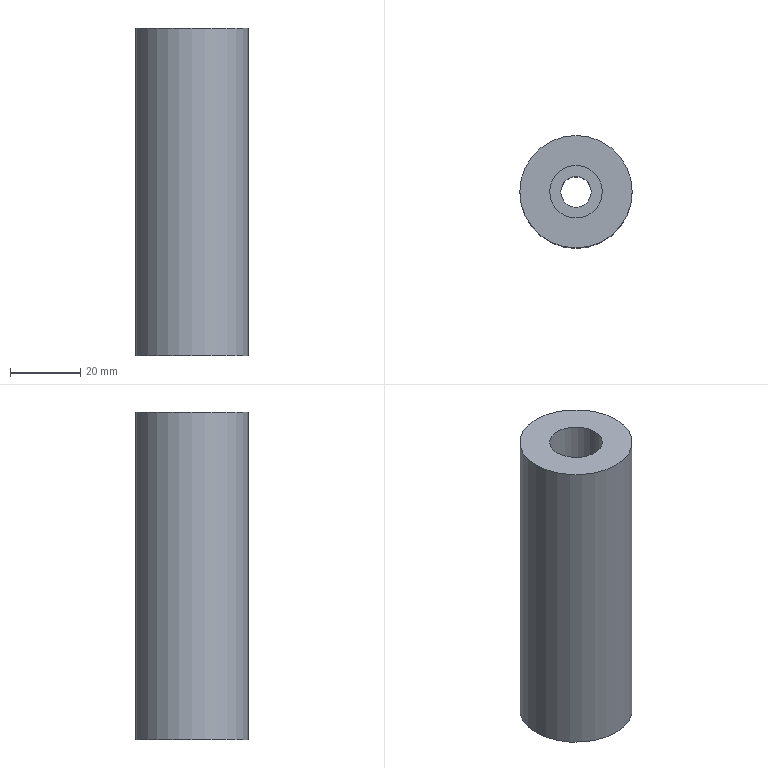Part | STEP file | 1_id1238_x_t | 1 solid | 6 faces | box 32 x 32 x 93.24 mm | volume 66514 mm3 | cylinder 3 | plane 3 | commonest cylinder face diameters 8.7 x1 15 x1 32 x1
STEP:
#1=CARTESIAN_POINT('',(0.,0.,0.));
#2=DIRECTION('',(0.,0.,1.));
#3=DIRECTION('',(1.,0.,0.));
#4=AXIS2_PLACEMENT_3D('',#1,#2,#3);
#5=CARTESIAN_POINT('',(906.425,64.5,-90.));
#6=VERTEX_POINT('',#5);
#7=CARTESIAN_POINT('',(874.425,64.5,-90.));
#8=VERTEX_POINT('',#7);
#9=CARTESIAN_POINT('',(890.425,64.5,-90.));
#10=DIRECTION('',(0.,0.,-1.));
#11=DIRECTION('',(-1.,0.,0.));
#12=AXIS2_PLACEMENT_3D('',#9,#10,#11);
#13=CIRCLE('',#12,16.);
#14=CARTESIAN_POINT('',(890.425,64.5,-46.76));
#15=DIRECTION('',(0.,0.,-1.));
#16=DIRECTION('',(1.,0.,0.));
#17=AXIS2_PLACEMENT_3D('',#14,#15,#16);
#18=CYLINDRICAL_SURFACE('',#17,16.);
#19=CARTESIAN_POINT('',(-3.142,43.24));
#20=DIRECTION('',(1.,0.));
#21=VECTOR('',#20,1.);
#22=LINE('',#19,#21);
#23=(GEOMETRIC_REPRESENTATION_CONTEXT(2)PARAMETRIC_REPRESENTATION_CONTEXT()REPRESENTATION_CONTEXT('',''));
#24=DEFINITIONAL_REPRESENTATION('',(#22),#23);
#25=PCURVE('',#18,#24);
#26=CARTESIAN_POINT('',(1119.226,213.819,-90.));
#27=DIRECTION('',(0.,0.,-1.));
#28=DIRECTION('',(0.,1.,0.));
#29=AXIS2_PLACEMENT_3D('',#26,#27,#28);
#30=PLANE('',#29);
#31=CARTESIAN_POINT('',(-149.319,-228.801));
#32=DIRECTION('',(0.,-1.));
#33=AXIS2_PLACEMENT_2D('',#31,#32);
#34=CIRCLE('',#33,16.);
#35=(GEOMETRIC_REPRESENTATION_CONTEXT(2)PARAMETRIC_REPRESENTATION_CONTEXT()REPRESENTATION_CONTEXT('',''));
#36=DEFINITIONAL_REPRESENTATION('',(#34),#35);
#37=PCURVE('',#30,#36);
#38=SURFACE_CURVE('',#13,(#25,#37),.PCURVE_S1.);
#39=EDGE_CURVE('',#6,#8,#38,.T.);
#40=ORIENTED_EDGE('',*,*,#39,.F.);
#41=CARTESIAN_POINT('',(906.425,64.5,3.24));
#42=VERTEX_POINT('',#41);
#43=CARTESIAN_POINT('',(906.425,64.5,3.24));
#44=CARTESIAN_POINT('',(906.425,64.5,-90.));
#45=B_SPLINE_CURVE_WITH_KNOTS('',1,(#43,#44),.UNSPECIFIED.,.F.,.F.,(2,2),(-50.,43.24),.PIECEWISE_BEZIER_KNOTS.);
#46=CARTESIAN_POINT('',(0.,0.));
#47=DIRECTION('',(0.,1.));
#48=VECTOR('',#47,1.);
#49=LINE('',#46,#48);
#50=(GEOMETRIC_REPRESENTATION_CONTEXT(2)PARAMETRIC_REPRESENTATION_CONTEXT()REPRESENTATION_CONTEXT('',''));
#51=DEFINITIONAL_REPRESENTATION('',(#49),#50);
#52=PCURVE('',#18,#51);
#53=CARTESIAN_POINT('',(6.283,0.));
#54=DIRECTION('',(0.,1.));
#55=VECTOR('',#54,1.);
#56=LINE('',#53,#55);
#57=(GEOMETRIC_REPRESENTATION_CONTEXT(2)PARAMETRIC_REPRESENTATION_CONTEXT()REPRESENTATION_CONTEXT('',''));
#58=DEFINITIONAL_REPRESENTATION('',(#56),#57);
#59=PCURVE('',#18,#58);
#60=SEAM_CURVE('',#45,(#52,#59),.PCURVE_S1.);
#61=EDGE_CURVE('',#42,#6,#60,.T.);
#62=ORIENTED_EDGE('',*,*,#61,.F.);
#63=CARTESIAN_POINT('',(890.425,64.5,3.24));
#64=DIRECTION('',(0.,0.,1.));
#65=DIRECTION('',(1.,0.,0.));
#66=AXIS2_PLACEMENT_3D('',#63,#64,#65);
#67=CIRCLE('',#66,16.);
#68=CARTESIAN_POINT('',(6.283,-50.));
#69=DIRECTION('',(-1.,0.));
#70=VECTOR('',#69,1.);
#71=LINE('',#68,#70);
#72=(GEOMETRIC_REPRESENTATION_CONTEXT(2)PARAMETRIC_REPRESENTATION_CONTEXT()REPRESENTATION_CONTEXT('',''));
#73=DEFINITIONAL_REPRESENTATION('',(#71),#72);
#74=PCURVE('',#18,#73);
#75=CARTESIAN_POINT('',(890.425,64.5,3.24));
#76=DIRECTION('',(0.,0.,-1.));
#77=DIRECTION('',(-1.,0.,0.));
#78=AXIS2_PLACEMENT_3D('',#75,#76,#77);
#79=PLANE('',#78);
#80=CARTESIAN_POINT('',(-16.,0.));
#81=CARTESIAN_POINT('',(-16.,27.713));
#82=CARTESIAN_POINT('',(8.,13.856));
#83=CARTESIAN_POINT('',(32.,0.));
#84=CARTESIAN_POINT('',(8.,-13.856));
#85=CARTESIAN_POINT('',(-16.,-27.713));
#86=CARTESIAN_POINT('',(-16.,0.));
#87=(BOUNDED_CURVE()B_SPLINE_CURVE(2,(#80,#81,#82,#83,#84,#85,#86),.UNSPECIFIED.,.T.,.F.)B_SPLINE_CURVE_WITH_KNOTS((1,2,2,2,2,1),(-2.094,0.,2.094,4.189,6.283,8.378),.UNSPECIFIED.)CURVE()GEOMETRIC_REPRESENTATION_ITEM()RATIONAL_B_SPLINE_CURVE((1.,0.5,1.,0.5,1.,0.5,1.))REPRESENTATION_ITEM(''));
#88=(GEOMETRIC_REPRESENTATION_CONTEXT(2)PARAMETRIC_REPRESENTATION_CONTEXT()REPRESENTATION_CONTEXT('',''));
#89=DEFINITIONAL_REPRESENTATION('',(#87),#88);
#90=PCURVE('',#79,#89);
#91=SURFACE_CURVE('',#67,(#74,#90),.PCURVE_S1.);
#92=EDGE_CURVE('',#42,#42,#91,.T.);
#93=ORIENTED_EDGE('',*,*,#92,.F.);
#94=ORIENTED_EDGE('',*,*,#61,.T.);
#95=CARTESIAN_POINT('',(890.425,64.5,-90.));
#96=DIRECTION('',(0.,0.,-1.));
#97=DIRECTION('',(-1.,0.,0.));
#98=AXIS2_PLACEMENT_3D('',#95,#96,#97);
#99=CIRCLE('',#98,16.);
#100=CARTESIAN_POINT('',(3.142,43.24));
#101=DIRECTION('',(1.,0.));
#102=VECTOR('',#101,1.);
#103=LINE('',#100,#102);
#104=(GEOMETRIC_REPRESENTATION_CONTEXT(2)PARAMETRIC_REPRESENTATION_CONTEXT()REPRESENTATION_CONTEXT('',''));
#105=DEFINITIONAL_REPRESENTATION('',(#103),#104);
#106=PCURVE('',#18,#105);
#107=CARTESIAN_POINT('',(-149.319,-228.801));
#108=DIRECTION('',(0.,-1.));
#109=AXIS2_PLACEMENT_2D('',#107,#108);
#110=CIRCLE('',#109,16.);
#111=(GEOMETRIC_REPRESENTATION_CONTEXT(2)PARAMETRIC_REPRESENTATION_CONTEXT()REPRESENTATION_CONTEXT('',''));
#112=DEFINITIONAL_REPRESENTATION('',(#110),#111);
#113=PCURVE('',#30,#112);
#114=SURFACE_CURVE('',#99,(#106,#113),.PCURVE_S1.);
#115=EDGE_CURVE('',#8,#6,#114,.T.);
#116=ORIENTED_EDGE('',*,*,#115,.F.);
#117=EDGE_LOOP('',(#40,#62,#93,#94,#116));
#118=FACE_BOUND('',#117,.T.);
#119=ADVANCED_FACE('',(#118),#18,.T.);
#120=ORIENTED_EDGE('',*,*,#115,.T.);
#121=ORIENTED_EDGE('',*,*,#39,.T.);
#122=EDGE_LOOP('',(#120,#121));
#123=FACE_BOUND('',#122,.T.);
#124=CARTESIAN_POINT('',(894.775,64.5,-90.));
#125=VERTEX_POINT('',#124);
#126=CARTESIAN_POINT('',(890.425,64.5,-90.));
#127=DIRECTION('',(0.,0.,1.));
#128=DIRECTION('',(1.,0.,0.));
#129=AXIS2_PLACEMENT_3D('',#126,#127,#128);
#130=CIRCLE('',#129,4.35);
#131=CARTESIAN_POINT('',(-149.319,-224.451));
#132=CARTESIAN_POINT('',(-141.785,-224.451));
#133=CARTESIAN_POINT('',(-145.552,-230.976));
#134=CARTESIAN_POINT('',(-149.319,-237.501));
#135=CARTESIAN_POINT('',(-153.086,-230.976));
#136=CARTESIAN_POINT('',(-156.854,-224.451));
#137=CARTESIAN_POINT('',(-149.319,-224.451));
#138=(BOUNDED_CURVE()B_SPLINE_CURVE(2,(#131,#132,#133,#134,#135,#136,#137),.UNSPECIFIED.,.T.,.F.)B_SPLINE_CURVE_WITH_KNOTS((1,2,2,2,2,1),(-2.094,0.,2.094,4.189,6.283,8.378),.UNSPECIFIED.)CURVE()GEOMETRIC_REPRESENTATION_ITEM()RATIONAL_B_SPLINE_CURVE((1.,0.5,1.,0.5,1.,0.5,1.))REPRESENTATION_ITEM(''));
#139=(GEOMETRIC_REPRESENTATION_CONTEXT(2)PARAMETRIC_REPRESENTATION_CONTEXT()REPRESENTATION_CONTEXT('',''));
#140=DEFINITIONAL_REPRESENTATION('',(#138),#139);
#141=PCURVE('',#30,#140);
#142=CARTESIAN_POINT('',(890.425,64.5,-47.26));
#143=DIRECTION('',(0.,0.,-1.));
#144=DIRECTION('',(1.,0.,0.));
#145=AXIS2_PLACEMENT_3D('',#142,#143,#144);
#146=CYLINDRICAL_SURFACE('',#145,4.35);
#147=CARTESIAN_POINT('',(6.283,42.74));
#148=DIRECTION('',(-1.,0.));
#149=VECTOR('',#148,1.);
#150=LINE('',#147,#149);
#151=(GEOMETRIC_REPRESENTATION_CONTEXT(2)PARAMETRIC_REPRESENTATION_CONTEXT()REPRESENTATION_CONTEXT('',''));
#152=DEFINITIONAL_REPRESENTATION('',(#150),#151);
#153=PCURVE('',#146,#152);
#154=SURFACE_CURVE('',#130,(#141,#153),.PCURVE_S1.);
#155=EDGE_CURVE('',#125,#125,#154,.T.);
#156=ORIENTED_EDGE('',*,*,#155,.T.);
#157=EDGE_LOOP('',(#156));
#158=FACE_BOUND('',#157,.T.);
#159=ADVANCED_FACE('',(#123,#158),#30,.T.);
#160=ORIENTED_EDGE('',*,*,#92,.T.);
#161=EDGE_LOOP('',(#160));
#162=FACE_BOUND('',#161,.T.);
#163=CARTESIAN_POINT('',(882.925,64.5,3.24));
#164=VERTEX_POINT('',#163);
#165=CARTESIAN_POINT('',(897.925,64.5,3.24));
#166=VERTEX_POINT('',#165);
#167=CARTESIAN_POINT('',(890.425,64.5,3.24));
#168=DIRECTION('',(0.,0.,-1.));
#169=DIRECTION('',(-1.,0.,0.));
#170=AXIS2_PLACEMENT_3D('',#167,#168,#169);
#171=CIRCLE('',#170,7.5);
#172=CARTESIAN_POINT('',(0.,0.));
#173=DIRECTION('',(1.,0.));
#174=AXIS2_PLACEMENT_2D('',#172,#173);
#175=CIRCLE('',#174,7.5);
#176=(GEOMETRIC_REPRESENTATION_CONTEXT(2)PARAMETRIC_REPRESENTATION_CONTEXT()REPRESENTATION_CONTEXT('',''));
#177=DEFINITIONAL_REPRESENTATION('',(#175),#176);
#178=PCURVE('',#79,#177);
#179=CARTESIAN_POINT('',(890.425,64.5,-9.76));
#180=DIRECTION('',(0.,0.,-1.));
#181=DIRECTION('',(1.,0.,0.));
#182=AXIS2_PLACEMENT_3D('',#179,#180,#181);
#183=CYLINDRICAL_SURFACE('',#182,7.5);
#184=CARTESIAN_POINT('',(3.142,-13.));
#185=DIRECTION('',(1.,0.));
#186=VECTOR('',#185,1.);
#187=LINE('',#184,#186);
#188=(GEOMETRIC_REPRESENTATION_CONTEXT(2)PARAMETRIC_REPRESENTATION_CONTEXT()REPRESENTATION_CONTEXT('',''));
#189=DEFINITIONAL_REPRESENTATION('',(#187),#188);
#190=PCURVE('',#183,#189);
#191=SURFACE_CURVE('',#171,(#178,#190),.PCURVE_S1.);
#192=EDGE_CURVE('',#164,#166,#191,.T.);
#193=ORIENTED_EDGE('',*,*,#192,.T.);
#194=CARTESIAN_POINT('',(890.425,64.5,3.24));
#195=DIRECTION('',(0.,0.,-1.));
#196=DIRECTION('',(-1.,0.,0.));
#197=AXIS2_PLACEMENT_3D('',#194,#195,#196);
#198=CIRCLE('',#197,7.5);
#199=CARTESIAN_POINT('',(0.,0.));
#200=DIRECTION('',(1.,0.));
#201=AXIS2_PLACEMENT_2D('',#199,#200);
#202=CIRCLE('',#201,7.5);
#203=(GEOMETRIC_REPRESENTATION_CONTEXT(2)PARAMETRIC_REPRESENTATION_CONTEXT()REPRESENTATION_CONTEXT('',''));
#204=DEFINITIONAL_REPRESENTATION('',(#202),#203);
#205=PCURVE('',#79,#204);
#206=CARTESIAN_POINT('',(-3.142,-13.));
#207=DIRECTION('',(1.,0.));
#208=VECTOR('',#207,1.);
#209=LINE('',#206,#208);
#210=(GEOMETRIC_REPRESENTATION_CONTEXT(2)PARAMETRIC_REPRESENTATION_CONTEXT()REPRESENTATION_CONTEXT('',''));
#211=DEFINITIONAL_REPRESENTATION('',(#209),#210);
#212=PCURVE('',#183,#211);
#213=SURFACE_CURVE('',#198,(#205,#212),.PCURVE_S1.);
#214=EDGE_CURVE('',#166,#164,#213,.T.);
#215=ORIENTED_EDGE('',*,*,#214,.T.);
#216=EDGE_LOOP('',(#193,#215));
#217=FACE_BOUND('',#216,.T.);
#218=ADVANCED_FACE('',(#162,#217),#79,.F.);
#219=CARTESIAN_POINT('',(897.925,64.5,-21.76));
#220=VERTEX_POINT('',#219);
#221=CARTESIAN_POINT('',(890.425,64.5,-21.76));
#222=DIRECTION('',(0.,0.,1.));
#223=DIRECTION('',(1.,0.,0.));
#224=AXIS2_PLACEMENT_3D('',#221,#222,#223);
#225=CIRCLE('',#224,7.5);
#226=CARTESIAN_POINT('',(6.283,12.));
#227=DIRECTION('',(-1.,0.));
#228=VECTOR('',#227,1.);
#229=LINE('',#226,#228);
#230=(GEOMETRIC_REPRESENTATION_CONTEXT(2)PARAMETRIC_REPRESENTATION_CONTEXT()REPRESENTATION_CONTEXT('',''));
#231=DEFINITIONAL_REPRESENTATION('',(#229),#230);
#232=PCURVE('',#183,#231);
#233=CARTESIAN_POINT('',(890.425,64.5,-21.76));
#234=DIRECTION('',(0.,0.,-1.));
#235=DIRECTION('',(-1.,0.,0.));
#236=AXIS2_PLACEMENT_3D('',#233,#234,#235);
#237=PLANE('',#236);
#238=CARTESIAN_POINT('',(-7.5,0.));
#239=CARTESIAN_POINT('',(-7.5,12.99));
#240=CARTESIAN_POINT('',(3.75,6.495));
#241=CARTESIAN_POINT('',(15.,0.));
#242=CARTESIAN_POINT('',(3.75,-6.495));
#243=CARTESIAN_POINT('',(-7.5,-12.99));
#244=CARTESIAN_POINT('',(-7.5,0.));
#245=(BOUNDED_CURVE()B_SPLINE_CURVE(2,(#238,#239,#240,#241,#242,#243,#244),.UNSPECIFIED.,.T.,.F.)B_SPLINE_CURVE_WITH_KNOTS((1,2,2,2,2,1),(-2.094,0.,2.094,4.189,6.283,8.378),.UNSPECIFIED.)CURVE()GEOMETRIC_REPRESENTATION_ITEM()RATIONAL_B_SPLINE_CURVE((1.,0.5,1.,0.5,1.,0.5,1.))REPRESENTATION_ITEM(''));
#246=(GEOMETRIC_REPRESENTATION_CONTEXT(2)PARAMETRIC_REPRESENTATION_CONTEXT()REPRESENTATION_CONTEXT('',''));
#247=DEFINITIONAL_REPRESENTATION('',(#245),#246);
#248=PCURVE('',#237,#247);
#249=SURFACE_CURVE('',#225,(#232,#248),.PCURVE_S1.);
#250=EDGE_CURVE('',#220,#220,#249,.T.);
#251=ORIENTED_EDGE('',*,*,#250,.T.);
#252=CARTESIAN_POINT('',(897.925,64.5,3.24));
#253=CARTESIAN_POINT('',(897.925,64.5,-21.76));
#254=B_SPLINE_CURVE_WITH_KNOTS('',1,(#252,#253),.UNSPECIFIED.,.F.,.F.,(2,2),(-13.,12.),.PIECEWISE_BEZIER_KNOTS.);
#255=CARTESIAN_POINT('',(0.,0.));
#256=DIRECTION('',(0.,1.));
#257=VECTOR('',#256,1.);
#258=LINE('',#255,#257);
#259=(GEOMETRIC_REPRESENTATION_CONTEXT(2)PARAMETRIC_REPRESENTATION_CONTEXT()REPRESENTATION_CONTEXT('',''));
#260=DEFINITIONAL_REPRESENTATION('',(#258),#259);
#261=PCURVE('',#183,#260);
#262=CARTESIAN_POINT('',(6.283,0.));
#263=DIRECTION('',(0.,1.));
#264=VECTOR('',#263,1.);
#265=LINE('',#262,#264);
#266=(GEOMETRIC_REPRESENTATION_CONTEXT(2)PARAMETRIC_REPRESENTATION_CONTEXT()REPRESENTATION_CONTEXT('',''));
#267=DEFINITIONAL_REPRESENTATION('',(#265),#266);
#268=PCURVE('',#183,#267);
#269=SEAM_CURVE('',#254,(#261,#268),.PCURVE_S1.);
#270=EDGE_CURVE('',#166,#220,#269,.T.);
#271=ORIENTED_EDGE('',*,*,#270,.F.);
#272=ORIENTED_EDGE('',*,*,#214,.T.);
#273=ORIENTED_EDGE('',*,*,#192,.T.);
#274=ORIENTED_EDGE('',*,*,#270,.T.);
#275=EDGE_LOOP('',(#251,#271,#272,#273,#274));
#276=FACE_BOUND('',#275,.F.);
#277=ADVANCED_FACE('',(#276),#183,.F.);
#278=ORIENTED_EDGE('',*,*,#250,.T.);
#279=EDGE_LOOP('',(#278));
#280=FACE_BOUND('',#279,.T.);
#281=CARTESIAN_POINT('',(894.775,64.5,-21.76));
#282=VERTEX_POINT('',#281);
#283=CARTESIAN_POINT('',(890.425,64.5,-21.76));
#284=DIRECTION('',(0.,0.,-1.));
#285=DIRECTION('',(1.,0.,0.));
#286=AXIS2_PLACEMENT_3D('',#283,#284,#285);
#287=CIRCLE('',#286,4.35);
#288=CARTESIAN_POINT('',(0.,0.));
#289=DIRECTION('',(-1.,0.));
#290=AXIS2_PLACEMENT_2D('',#288,#289);
#291=CIRCLE('',#290,4.35);
#292=(GEOMETRIC_REPRESENTATION_CONTEXT(2)PARAMETRIC_REPRESENTATION_CONTEXT()REPRESENTATION_CONTEXT('',''));
#293=DEFINITIONAL_REPRESENTATION('',(#291),#292);
#294=PCURVE('',#237,#293);
#295=CARTESIAN_POINT('',(0.,-25.5));
#296=DIRECTION('',(1.,0.));
#297=VECTOR('',#296,1.);
#298=LINE('',#295,#297);
#299=(GEOMETRIC_REPRESENTATION_CONTEXT(2)PARAMETRIC_REPRESENTATION_CONTEXT()REPRESENTATION_CONTEXT('',''));
#300=DEFINITIONAL_REPRESENTATION('',(#298),#299);
#301=PCURVE('',#146,#300);
#302=SURFACE_CURVE('',#287,(#294,#301),.PCURVE_S1.);
#303=EDGE_CURVE('',#282,#282,#302,.T.);
#304=ORIENTED_EDGE('',*,*,#303,.T.);
#305=EDGE_LOOP('',(#304));
#306=FACE_BOUND('',#305,.T.);
#307=ADVANCED_FACE('',(#280,#306),#237,.F.);
#308=ORIENTED_EDGE('',*,*,#155,.T.);
#309=CARTESIAN_POINT('',(894.775,64.5,-21.76));
#310=CARTESIAN_POINT('',(894.775,64.5,-90.));
#311=B_SPLINE_CURVE_WITH_KNOTS('',1,(#309,#310),.UNSPECIFIED.,.F.,.F.,(2,2),(-25.5,42.74),.PIECEWISE_BEZIER_KNOTS.);
#312=CARTESIAN_POINT('',(0.,0.));
#313=DIRECTION('',(0.,1.));
#314=VECTOR('',#313,1.);
#315=LINE('',#312,#314);
#316=(GEOMETRIC_REPRESENTATION_CONTEXT(2)PARAMETRIC_REPRESENTATION_CONTEXT()REPRESENTATION_CONTEXT('',''));
#317=DEFINITIONAL_REPRESENTATION('',(#315),#316);
#318=PCURVE('',#146,#317);
#319=CARTESIAN_POINT('',(6.283,0.));
#320=DIRECTION('',(0.,1.));
#321=VECTOR('',#320,1.);
#322=LINE('',#319,#321);
#323=(GEOMETRIC_REPRESENTATION_CONTEXT(2)PARAMETRIC_REPRESENTATION_CONTEXT()REPRESENTATION_CONTEXT('',''));
#324=DEFINITIONAL_REPRESENTATION('',(#322),#323);
#325=PCURVE('',#146,#324);
#326=SEAM_CURVE('',#311,(#318,#325),.PCURVE_S1.);
#327=EDGE_CURVE('',#282,#125,#326,.T.);
#328=ORIENTED_EDGE('',*,*,#327,.F.);
#329=ORIENTED_EDGE('',*,*,#303,.T.);
#330=ORIENTED_EDGE('',*,*,#327,.T.);
#331=EDGE_LOOP('',(#308,#328,#329,#330));
#332=FACE_BOUND('',#331,.F.);
#333=ADVANCED_FACE('',(#332),#146,.F.);
#334=CLOSED_SHELL('',(#119,#159,#218,#277,#307,#333));
#335=MANIFOLD_SOLID_BREP('',#334);
#336=(LENGTH_UNIT()NAMED_UNIT(*)SI_UNIT(.MILLI.,.METRE.));
#337=UNCERTAINTY_MEASURE_WITH_UNIT(LENGTH_MEASURE(0.000005),#336,'','');
#338=(NAMED_UNIT(*)PLANE_ANGLE_UNIT()SI_UNIT($,.RADIAN.));
#339=(NAMED_UNIT(*)SI_UNIT($,.STERADIAN.)SOLID_ANGLE_UNIT());
#340=(GEOMETRIC_REPRESENTATION_CONTEXT(3)GLOBAL_UNCERTAINTY_ASSIGNED_CONTEXT((#337))GLOBAL_UNIT_ASSIGNED_CONTEXT((#336,#338,#339))REPRESENTATION_CONTEXT('',''));
#341=ADVANCED_BREP_SHAPE_REPRESENTATION('',(#4,#335),#340);